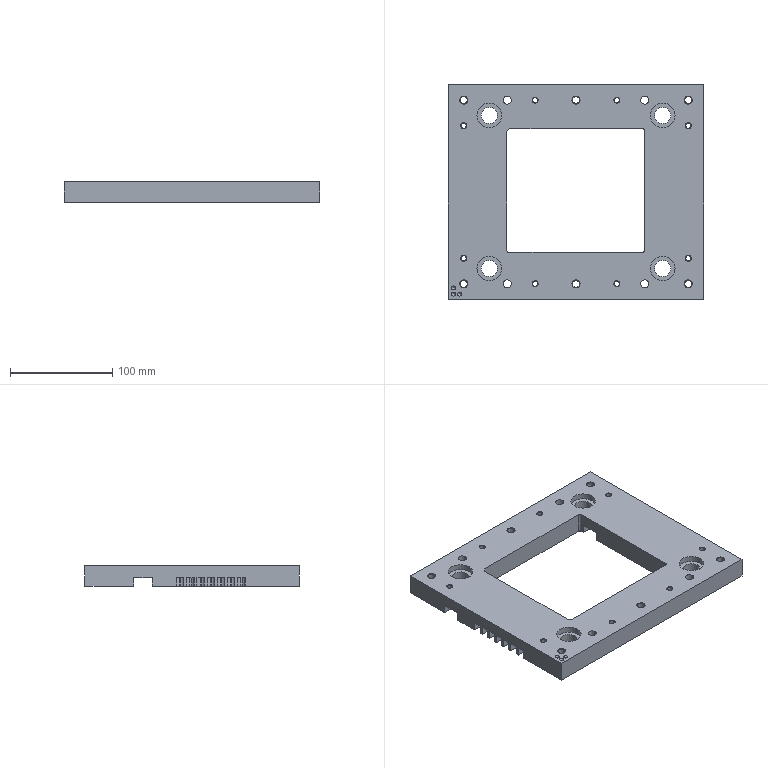Part | STEP file | 200 mesh_id2090 | 1 solid | 188 faces | box 250 x 210 x 20 mm | volume 615513 mm3 | plane 90 | cylinder 67 | cone 31 | commonest cylinder face diameters 6 x28 5 x8 6.8 x6 14 x6 8 x4 12 x4